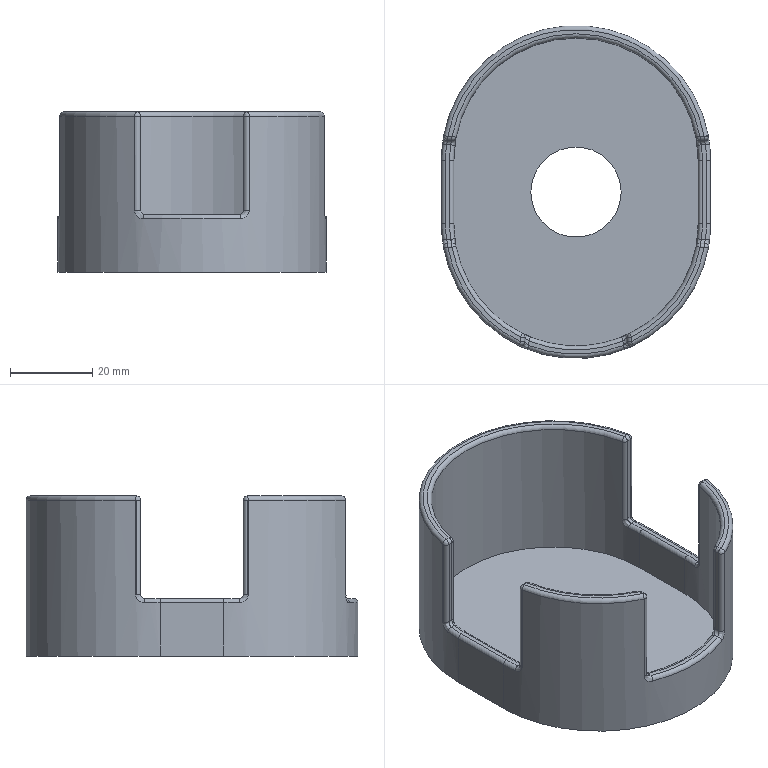Part | SolidWorks | features ICE 3, Extrusion 1, Fillet 1, Shell 1 | 1 solid | 96 faces | box 65.5 x 81 x 39 mm | volume 30712 mm3 | cylinder 36 | plane 18 | torus 16 | sphere 14 | spline 12 | commonest cylinder face diameters 2 x30 22 x2 59.5 x2 65.5 x2